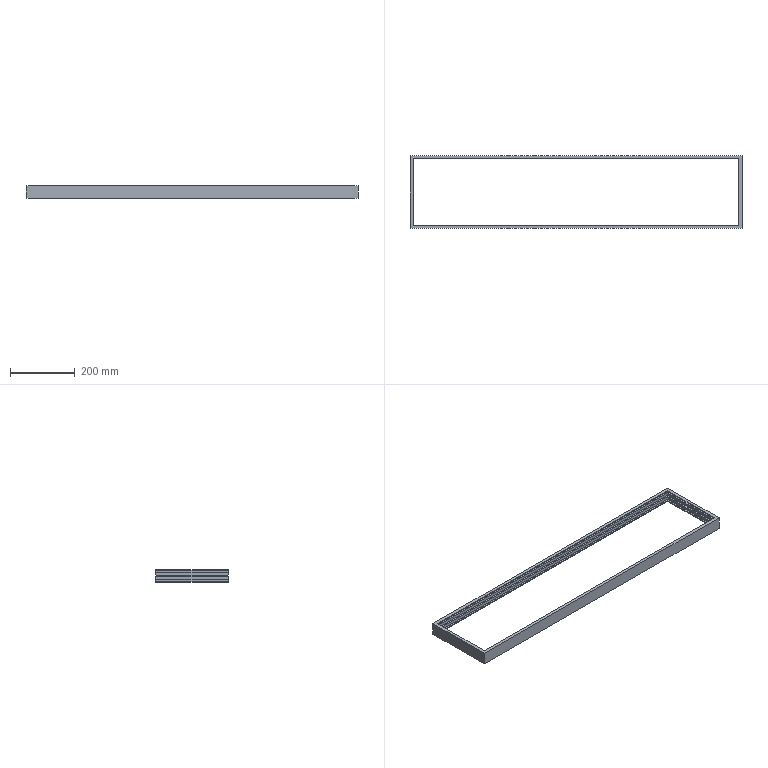Part | STEP file | 1 solid | 40 faces | box 1025 x 225 x 40 mm | volume 726960 mm3 | plane 40